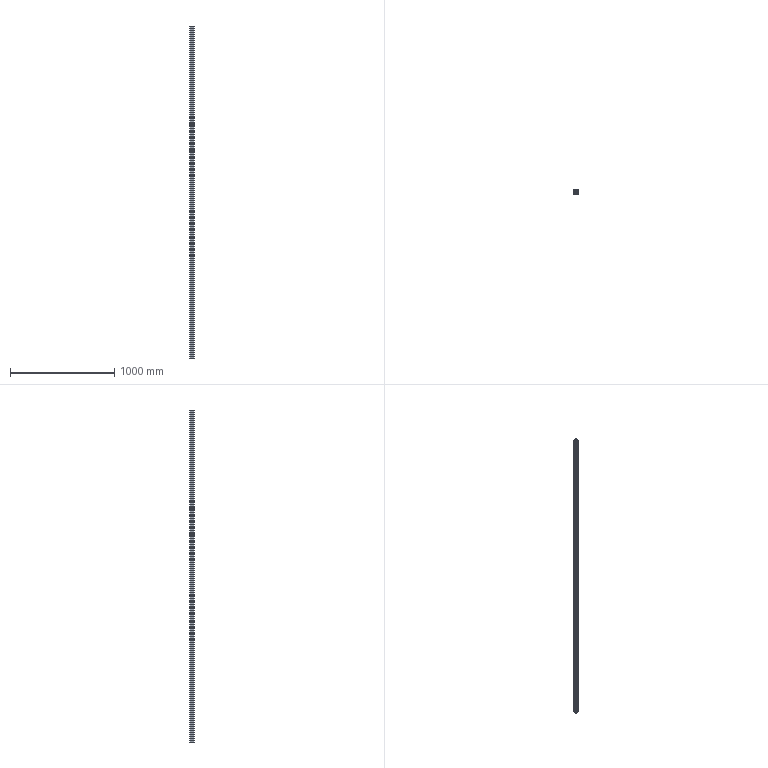Part | STEP file | 40x40-3180 | 1 solid | 88 faces | box 40 x 40 x 3180 mm | volume 2238551 mm3 | plane 78 | cylinder 10 | commonest cylinder face diameters 4 x4 10 x4 6.8 x2